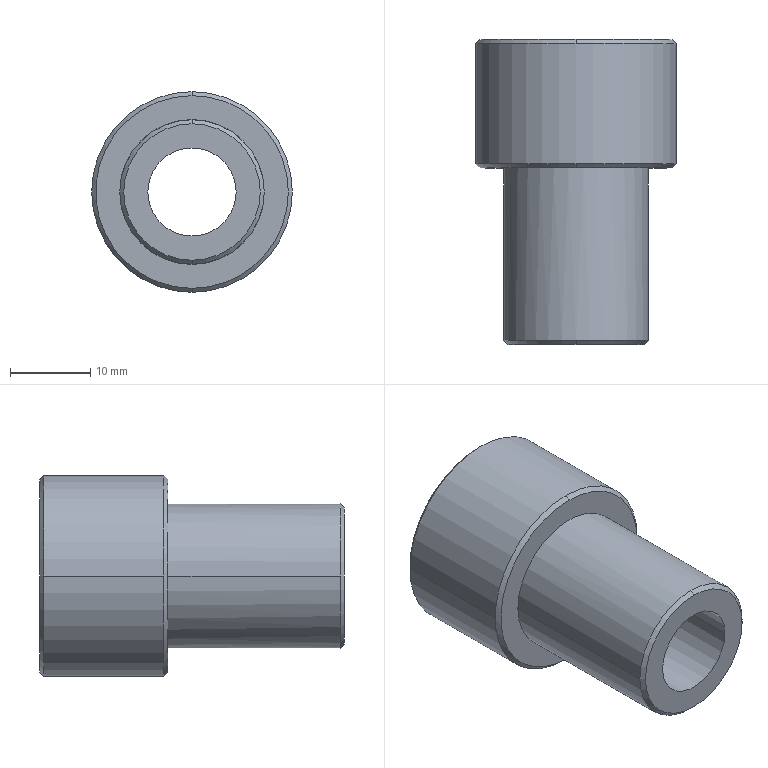Part | Creo | 1 solid | 20 faces | box 25 x 38 x 25 mm | volume 8054 mm3 | cylinder 8 | cone 8 | plane 4 | commonest cylinder face diameters 18 x4 11 x2 25 x2
STEP:
#1=CARTESIAN_POINT('',(-198.,355.995,-140.));
#2=VERTEX_POINT('',#1);
#3=CARTESIAN_POINT('',(-187.,355.995,-140.));
#4=VERTEX_POINT('',#3);
#5=CARTESIAN_POINT('',(-192.5,355.995,-140.));
#6=DIRECTION('',(0.,-1.,0.));
#7=DIRECTION('',(-1.,0.,0.));
#8=AXIS2_PLACEMENT_3D('',#5,#6,#7);
#9=CIRCLE('',#8,5.5);
#10=EDGE_CURVE('',#2,#4,#9,.T.);
#11=ORIENTED_EDGE('',*,*,#10,.T.);
#12=CARTESIAN_POINT('',(-187.,328.995,-140.));
#13=VERTEX_POINT('',#12);
#14=CARTESIAN_POINT('',(-187.,328.995,-140.));
#15=DIRECTION('',(0.,1.,0.));
#16=VECTOR('',#15,27.);
#17=LINE('',#14,#16);
#18=EDGE_CURVE('',#13,#4,#17,.T.);
#19=ORIENTED_EDGE('',*,*,#18,.F.);
#20=CARTESIAN_POINT('',(-198.,328.995,-140.));
#21=VERTEX_POINT('',#20);
#22=CARTESIAN_POINT('',(-192.5,328.995,-140.));
#23=DIRECTION('',(0.,1.,0.));
#24=DIRECTION('',(1.,0.,0.));
#25=AXIS2_PLACEMENT_3D('',#22,#23,#24);
#26=CIRCLE('',#25,5.5);
#27=EDGE_CURVE('',#13,#21,#26,.T.);
#28=ORIENTED_EDGE('',*,*,#27,.T.);
#29=CARTESIAN_POINT('',(-198.,328.995,-140.));
#30=DIRECTION('',(0.,1.,0.));
#31=VECTOR('',#30,27.);
#32=LINE('',#29,#31);
#33=EDGE_CURVE('',#21,#2,#32,.T.);
#34=ORIENTED_EDGE('',*,*,#33,.T.);
#35=EDGE_LOOP('',(#11,#19,#28,#34));
#36=FACE_OUTER_BOUND('',#35,.F.);
#37=CARTESIAN_POINT('',(-192.5,355.995,-140.));
#38=DIRECTION('',(0.,1.,0.));
#39=DIRECTION('',(1.,0.,0.));
#40=AXIS2_PLACEMENT_3D('',#37,#38,#39);
#41=CYLINDRICAL_SURFACE('',#40,5.5);
#42=ADVANCED_FACE('',(#36),#41,.F.);
#43=CARTESIAN_POINT('',(-183.5,355.995,-140.));
#44=VERTEX_POINT('',#43);
#45=CARTESIAN_POINT('',(-201.5,355.995,-140.));
#46=VERTEX_POINT('',#45);
#47=CARTESIAN_POINT('',(-192.5,355.995,-140.));
#48=DIRECTION('',(0.,1.,0.));
#49=DIRECTION('',(1.,0.,0.));
#50=AXIS2_PLACEMENT_3D('',#47,#48,#49);
#51=CIRCLE('',#50,9.);
#52=EDGE_CURVE('',#44,#46,#51,.T.);
#53=ORIENTED_EDGE('',*,*,#52,.F.);
#54=CARTESIAN_POINT('',(-192.5,355.995,-140.));
#55=DIRECTION('',(0.,1.,0.));
#56=DIRECTION('',(-1.,0.,0.));
#57=AXIS2_PLACEMENT_3D('',#54,#55,#56);
#58=CIRCLE('',#57,9.);
#59=EDGE_CURVE('',#46,#44,#58,.T.);
#60=ORIENTED_EDGE('',*,*,#59,.F.);
#61=EDGE_LOOP('',(#53,#60));
#62=FACE_OUTER_BOUND('',#61,.F.);
#63=CARTESIAN_POINT('',(-192.5,355.995,-140.));
#64=DIRECTION('',(0.,-1.,0.));
#65=DIRECTION('',(1.,0.,0.));
#66=AXIS2_PLACEMENT_3D('',#63,#64,#65);
#67=CIRCLE('',#66,5.5);
#68=EDGE_CURVE('',#4,#2,#67,.T.);
#69=ORIENTED_EDGE('',*,*,#68,.F.);
#70=ORIENTED_EDGE('',*,*,#10,.F.);
#71=EDGE_LOOP('',(#69,#70));
#72=FACE_BOUND('',#71,.F.);
#73=CARTESIAN_POINT('',(-192.5,355.995,-140.));
#74=DIRECTION('',(0.,-1.,0.));
#75=DIRECTION('',(1.,0.,0.));
#76=AXIS2_PLACEMENT_3D('',#73,#74,#75);
#77=PLANE('',#76);
#78=ADVANCED_FACE('',(#62,#72),#77,.F.);
#79=ORIENTED_EDGE('',*,*,#68,.T.);
#80=ORIENTED_EDGE('',*,*,#33,.F.);
#81=CARTESIAN_POINT('',(-192.5,328.995,-140.));
#82=DIRECTION('',(0.,1.,0.));
#83=DIRECTION('',(-1.,0.,0.));
#84=AXIS2_PLACEMENT_3D('',#81,#82,#83);
#85=CIRCLE('',#84,5.5);
#86=EDGE_CURVE('',#21,#13,#85,.T.);
#87=ORIENTED_EDGE('',*,*,#86,.T.);
#88=ORIENTED_EDGE('',*,*,#18,.T.);
#89=EDGE_LOOP('',(#79,#80,#87,#88));
#90=FACE_OUTER_BOUND('',#89,.F.);
#91=CARTESIAN_POINT('',(-192.5,355.995,-140.));
#92=DIRECTION('',(0.,1.,0.));
#93=DIRECTION('',(1.,0.,0.));
#94=AXIS2_PLACEMENT_3D('',#91,#92,#93);
#95=CYLINDRICAL_SURFACE('',#94,5.5);
#96=ADVANCED_FACE('',(#90),#95,.F.);
#97=CARTESIAN_POINT('',(-201.,328.995,-140.));
#98=VERTEX_POINT('',#97);
#99=CARTESIAN_POINT('',(-192.5,328.995,-148.5));
#100=VERTEX_POINT('',#99);
#101=CARTESIAN_POINT('',(-192.5,328.995,-140.));
#102=DIRECTION('',(0.,-1.,0.));
#103=DIRECTION('',(-1.,0.,0.));
#104=AXIS2_PLACEMENT_3D('',#101,#102,#103);
#105=CIRCLE('',#104,8.5);
#106=EDGE_CURVE('',#98,#100,#105,.T.);
#107=ORIENTED_EDGE('',*,*,#106,.F.);
#108=CARTESIAN_POINT('',(-192.5,328.995,-131.5));
#109=VERTEX_POINT('',#108);
#110=CARTESIAN_POINT('',(-192.5,328.995,-140.));
#111=DIRECTION('',(0.,-1.,0.));
#112=DIRECTION('',(0.,0.,1.));
#113=AXIS2_PLACEMENT_3D('',#110,#111,#112);
#114=CIRCLE('',#113,8.5);
#115=EDGE_CURVE('',#109,#98,#114,.T.);
#116=ORIENTED_EDGE('',*,*,#115,.F.);
#117=CARTESIAN_POINT('',(-184.,328.995,-140.));
#118=VERTEX_POINT('',#117);
#119=CARTESIAN_POINT('',(-192.5,328.995,-140.));
#120=DIRECTION('',(0.,-1.,0.));
#121=DIRECTION('',(1.,0.,0.));
#122=AXIS2_PLACEMENT_3D('',#119,#120,#121);
#123=CIRCLE('',#122,8.5);
#124=EDGE_CURVE('',#118,#109,#123,.T.);
#125=ORIENTED_EDGE('',*,*,#124,.F.);
#126=CARTESIAN_POINT('',(-192.5,328.995,-140.));
#127=DIRECTION('',(0.,-1.,0.));
#128=DIRECTION('',(0.,0.,-1.));
#129=AXIS2_PLACEMENT_3D('',#126,#127,#128);
#130=CIRCLE('',#129,8.5);
#131=EDGE_CURVE('',#100,#118,#130,.T.);
#132=ORIENTED_EDGE('',*,*,#131,.F.);
#133=EDGE_LOOP('',(#107,#116,#125,#132));
#134=FACE_OUTER_BOUND('',#133,.F.);
#135=ORIENTED_EDGE('',*,*,#27,.F.);
#136=ORIENTED_EDGE('',*,*,#86,.F.);
#137=EDGE_LOOP('',(#135,#136));
#138=FACE_BOUND('',#137,.F.);
#139=CARTESIAN_POINT('',(-232.5,328.995,-10.));
#140=DIRECTION('',(0.,-1.,0.));
#141=DIRECTION('',(1.,0.,0.));
#142=AXIS2_PLACEMENT_3D('',#139,#140,#141);
#143=PLANE('',#142);
#144=ADVANCED_FACE('',(#134,#138),#143,.T.);
#145=CARTESIAN_POINT('',(-201.5,329.495,-140.));
#146=VERTEX_POINT('',#145);
#147=CARTESIAN_POINT('',(-192.5,329.495,-149.));
#148=VERTEX_POINT('',#147);
#149=CARTESIAN_POINT('',(-192.5,329.495,-140.));
#150=DIRECTION('',(0.,-1.,0.));
#151=DIRECTION('',(-1.,0.,0.));
#152=AXIS2_PLACEMENT_3D('',#149,#150,#151);
#153=CIRCLE('',#152,9.);
#154=EDGE_CURVE('',#146,#148,#153,.T.);
#155=ORIENTED_EDGE('',*,*,#154,.F.);
#156=CARTESIAN_POINT('',(-192.5,329.495,-131.));
#157=VERTEX_POINT('',#156);
#158=CARTESIAN_POINT('',(-192.5,329.495,-140.));
#159=DIRECTION('',(0.,-1.,0.));
#160=DIRECTION('',(0.,0.,1.));
#161=AXIS2_PLACEMENT_3D('',#158,#159,#160);
#162=CIRCLE('',#161,9.);
#163=EDGE_CURVE('',#157,#146,#162,.T.);
#164=ORIENTED_EDGE('',*,*,#163,.F.);
#165=CARTESIAN_POINT('',(-192.5,328.995,-131.5));
#166=DIRECTION('',(0.,0.7071,0.7071));
#167=VECTOR('',#166,0.7071);
#168=LINE('',#165,#167);
#169=EDGE_CURVE('',#109,#157,#168,.T.);
#170=ORIENTED_EDGE('',*,*,#169,.F.);
#171=ORIENTED_EDGE('',*,*,#115,.T.);
#172=ORIENTED_EDGE('',*,*,#106,.T.);
#173=CARTESIAN_POINT('',(-192.5,328.995,-148.5));
#174=DIRECTION('',(0.,0.7071,-0.7071));
#175=VECTOR('',#174,0.7071);
#176=LINE('',#173,#175);
#177=EDGE_CURVE('',#100,#148,#176,.T.);
#178=ORIENTED_EDGE('',*,*,#177,.T.);
#179=EDGE_LOOP('',(#155,#164,#170,#171,#172,#178));
#180=FACE_OUTER_BOUND('',#179,.F.);
#181=CARTESIAN_POINT('',(-192.5,329.245,-140.));
#182=DIRECTION('',(0.,1.,0.));
#183=DIRECTION('',(0.,0.,-1.));
#184=AXIS2_PLACEMENT_3D('',#181,#182,#183);
#185=CONICAL_SURFACE('',#184,8.75,45.);
#186=ADVANCED_FACE('',(#180),#185,.T.);
#187=CARTESIAN_POINT('',(-183.5,329.495,-140.));
#188=VERTEX_POINT('',#187);
#189=CARTESIAN_POINT('',(-192.5,329.495,-140.));
#190=DIRECTION('',(0.,-1.,0.));
#191=DIRECTION('',(0.,0.,-1.));
#192=AXIS2_PLACEMENT_3D('',#189,#190,#191);
#193=CIRCLE('',#192,9.);
#194=EDGE_CURVE('',#148,#188,#193,.T.);
#195=ORIENTED_EDGE('',*,*,#194,.T.);
#196=CARTESIAN_POINT('',(-183.5,350.995,-140.));
#197=VERTEX_POINT('',#196);
#198=CARTESIAN_POINT('',(-183.5,350.995,-140.));
#199=DIRECTION('',(0.,-1.,0.));
#200=VECTOR('',#199,21.5);
#201=LINE('',#198,#200);
#202=EDGE_CURVE('',#197,#188,#201,.T.);
#203=ORIENTED_EDGE('',*,*,#202,.F.);
#204=CARTESIAN_POINT('',(-201.5,350.995,-140.));
#205=VERTEX_POINT('',#204);
#206=CARTESIAN_POINT('',(-192.5,350.995,-140.));
#207=DIRECTION('',(0.,1.,0.));
#208=DIRECTION('',(1.,0.,0.));
#209=AXIS2_PLACEMENT_3D('',#206,#207,#208);
#210=CIRCLE('',#209,9.);
#211=EDGE_CURVE('',#197,#205,#210,.T.);
#212=ORIENTED_EDGE('',*,*,#211,.T.);
#213=CARTESIAN_POINT('',(-201.5,350.995,-140.));
#214=DIRECTION('',(0.,-1.,0.));
#215=VECTOR('',#214,21.5);
#216=LINE('',#213,#215);
#217=EDGE_CURVE('',#205,#146,#216,.T.);
#218=ORIENTED_EDGE('',*,*,#217,.T.);
#219=ORIENTED_EDGE('',*,*,#154,.T.);
#220=EDGE_LOOP('',(#195,#203,#212,#218,#219));
#221=FACE_OUTER_BOUND('',#220,.F.);
#222=CARTESIAN_POINT('',(-192.5,331.995,-140.));
#223=DIRECTION('',(0.,-1.,0.));
#224=DIRECTION('',(1.,0.,0.));
#225=AXIS2_PLACEMENT_3D('',#222,#223,#224);
#226=CYLINDRICAL_SURFACE('',#225,9.);
#227=ADVANCED_FACE('',(#221),#226,.T.);
#228=ORIENTED_EDGE('',*,*,#194,.F.);
#229=ORIENTED_EDGE('',*,*,#177,.F.);
#230=ORIENTED_EDGE('',*,*,#131,.T.);
#231=ORIENTED_EDGE('',*,*,#124,.T.);
#232=ORIENTED_EDGE('',*,*,#169,.T.);
#233=CARTESIAN_POINT('',(-192.5,329.495,-140.));
#234=DIRECTION('',(0.,-1.,0.));
#235=DIRECTION('',(1.,0.,0.));
#236=AXIS2_PLACEMENT_3D('',#233,#234,#235);
#237=CIRCLE('',#236,9.);
#238=EDGE_CURVE('',#188,#157,#237,.T.);
#239=ORIENTED_EDGE('',*,*,#238,.F.);
#240=EDGE_LOOP('',(#228,#229,#230,#231,#232,#239));
#241=FACE_OUTER_BOUND('',#240,.F.);
#242=CARTESIAN_POINT('',(-192.5,329.245,-140.));
#243=DIRECTION('',(0.,1.,0.));
#244=DIRECTION('',(0.,0.,-1.));
#245=AXIS2_PLACEMENT_3D('',#242,#243,#244);
#246=CONICAL_SURFACE('',#245,8.75,45.);
#247=ADVANCED_FACE('',(#241),#246,.T.);
#248=ORIENTED_EDGE('',*,*,#163,.T.);
#249=ORIENTED_EDGE('',*,*,#217,.F.);
#250=CARTESIAN_POINT('',(-192.5,350.995,-140.));
#251=DIRECTION('',(0.,1.,0.));
#252=DIRECTION('',(-1.,0.,0.));
#253=AXIS2_PLACEMENT_3D('',#250,#251,#252);
#254=CIRCLE('',#253,9.);
#255=EDGE_CURVE('',#205,#197,#254,.T.);
#256=ORIENTED_EDGE('',*,*,#255,.T.);
#257=ORIENTED_EDGE('',*,*,#202,.T.);
#258=ORIENTED_EDGE('',*,*,#238,.T.);
#259=EDGE_LOOP('',(#248,#249,#256,#257,#258));
#260=FACE_OUTER_BOUND('',#259,.F.);
#261=CARTESIAN_POINT('',(-192.5,331.995,-140.));
#262=DIRECTION('',(0.,-1.,0.));
#263=DIRECTION('',(1.,0.,0.));
#264=AXIS2_PLACEMENT_3D('',#261,#262,#263);
#265=CYLINDRICAL_SURFACE('',#264,9.);
#266=ADVANCED_FACE('',(#260),#265,.T.);
#267=CARTESIAN_POINT('',(-180.5,350.995,-140.));
#268=VERTEX_POINT('',#267);
#269=CARTESIAN_POINT('',(-192.5,350.995,-128.));
#270=VERTEX_POINT('',#269);
#271=CARTESIAN_POINT('',(-192.5,350.995,-140.));
#272=DIRECTION('',(0.,-1.,0.));
#273=DIRECTION('',(1.,0.,0.));
#274=AXIS2_PLACEMENT_3D('',#271,#272,#273);
#275=CIRCLE('',#274,12.);
#276=EDGE_CURVE('',#268,#270,#275,.T.);
#277=ORIENTED_EDGE('',*,*,#276,.F.);
#278=CARTESIAN_POINT('',(-192.5,350.995,-152.));
#279=VERTEX_POINT('',#278);
#280=CARTESIAN_POINT('',(-192.5,350.995,-140.));
#281=DIRECTION('',(0.,-1.,0.));
#282=DIRECTION('',(0.,0.,-1.));
#283=AXIS2_PLACEMENT_3D('',#280,#281,#282);
#284=CIRCLE('',#283,12.);
#285=EDGE_CURVE('',#279,#268,#284,.T.);
#286=ORIENTED_EDGE('',*,*,#285,.F.);
#287=CARTESIAN_POINT('',(-192.5,350.995,-140.));
#288=DIRECTION('',(0.,-1.,0.));
#289=DIRECTION('',(0.,0.,1.));
#290=AXIS2_PLACEMENT_3D('',#287,#288,#289);
#291=CIRCLE('',#290,12.);
#292=EDGE_CURVE('',#270,#279,#291,.T.);
#293=ORIENTED_EDGE('',*,*,#292,.F.);
#294=EDGE_LOOP('',(#277,#286,#293));
#295=FACE_OUTER_BOUND('',#294,.F.);
#296=ORIENTED_EDGE('',*,*,#255,.F.);
#297=ORIENTED_EDGE('',*,*,#211,.F.);
#298=EDGE_LOOP('',(#296,#297));
#299=FACE_BOUND('',#298,.F.);
#300=CARTESIAN_POINT('',(-232.5,350.995,-10.));
#301=DIRECTION('',(0.,-1.,0.));
#302=DIRECTION('',(1.,0.,0.));
#303=AXIS2_PLACEMENT_3D('',#300,#301,#302);
#304=PLANE('',#303);
#305=ADVANCED_FACE('',(#295,#299),#304,.T.);
#306=CARTESIAN_POINT('',(-180.,351.495,-140.));
#307=VERTEX_POINT('',#306);
#308=CARTESIAN_POINT('',(-192.5,351.495,-127.5));
#309=VERTEX_POINT('',#308);
#310=CARTESIAN_POINT('',(-192.5,351.495,-140.));
#311=DIRECTION('',(0.,-1.,0.));
#312=DIRECTION('',(1.,0.,0.));
#313=AXIS2_PLACEMENT_3D('',#310,#311,#312);
#314=CIRCLE('',#313,12.5);
#315=EDGE_CURVE('',#307,#309,#314,.T.);
#316=ORIENTED_EDGE('',*,*,#315,.F.);
#317=CARTESIAN_POINT('',(-192.5,351.495,-152.5));
#318=VERTEX_POINT('',#317);
#319=CARTESIAN_POINT('',(-192.5,351.495,-140.));
#320=DIRECTION('',(0.,-1.,0.));
#321=DIRECTION('',(0.,0.,-1.));
#322=AXIS2_PLACEMENT_3D('',#319,#320,#321);
#323=CIRCLE('',#322,12.5);
#324=EDGE_CURVE('',#318,#307,#323,.T.);
#325=ORIENTED_EDGE('',*,*,#324,.F.);
#326=CARTESIAN_POINT('',(-192.5,350.995,-152.));
#327=DIRECTION('',(0.,0.7071,-0.7071));
#328=VECTOR('',#327,0.7071);
#329=LINE('',#326,#328);
#330=EDGE_CURVE('',#279,#318,#329,.T.);
#331=ORIENTED_EDGE('',*,*,#330,.F.);
#332=ORIENTED_EDGE('',*,*,#285,.T.);
#333=ORIENTED_EDGE('',*,*,#276,.T.);
#334=CARTESIAN_POINT('',(-192.5,350.995,-128.));
#335=DIRECTION('',(0.,0.7071,0.7071));
#336=VECTOR('',#335,0.7071);
#337=LINE('',#334,#336);
#338=EDGE_CURVE('',#270,#309,#337,.T.);
#339=ORIENTED_EDGE('',*,*,#338,.T.);
#340=EDGE_LOOP('',(#316,#325,#331,#332,#333,#339));
#341=FACE_OUTER_BOUND('',#340,.F.);
#342=CARTESIAN_POINT('',(-192.5,351.245,-140.));
#343=DIRECTION('',(0.,1.,0.));
#344=DIRECTION('',(0.,0.,-1.));
#345=AXIS2_PLACEMENT_3D('',#342,#343,#344);
#346=CONICAL_SURFACE('',#345,12.25,45.);
#347=ADVANCED_FACE('',(#341),#346,.T.);
#348=CARTESIAN_POINT('',(-205.,351.495,-140.));
#349=VERTEX_POINT('',#348);
#350=CARTESIAN_POINT('',(-192.5,351.495,-140.));
#351=DIRECTION('',(0.,-1.,0.));
#352=DIRECTION('',(0.,0.,1.));
#353=AXIS2_PLACEMENT_3D('',#350,#351,#352);
#354=CIRCLE('',#353,12.5);
#355=EDGE_CURVE('',#309,#349,#354,.T.);
#356=ORIENTED_EDGE('',*,*,#355,.T.);
#357=CARTESIAN_POINT('',(-205.,366.495,-140.));
#358=VERTEX_POINT('',#357);
#359=CARTESIAN_POINT('',(-205.,366.495,-140.));
#360=DIRECTION('',(0.,-1.,0.));
#361=VECTOR('',#360,15.);
#362=LINE('',#359,#361);
#363=EDGE_CURVE('',#358,#349,#362,.T.);
#364=ORIENTED_EDGE('',*,*,#363,.F.);
#365=CARTESIAN_POINT('',(-192.5,366.495,-127.5));
#366=VERTEX_POINT('',#365);
#367=CARTESIAN_POINT('',(-192.5,366.495,-140.));
#368=DIRECTION('',(0.,1.,0.));
#369=DIRECTION('',(-1.,0.,0.));
#370=AXIS2_PLACEMENT_3D('',#367,#368,#369);
#371=CIRCLE('',#370,12.5);
#372=EDGE_CURVE('',#358,#366,#371,.T.);
#373=ORIENTED_EDGE('',*,*,#372,.T.);
#374=CARTESIAN_POINT('',(-180.,366.495,-140.));
#375=VERTEX_POINT('',#374);
#376=CARTESIAN_POINT('',(-192.5,366.495,-140.));
#377=DIRECTION('',(0.,1.,0.));
#378=DIRECTION('',(0.,0.,1.));
#379=AXIS2_PLACEMENT_3D('',#376,#377,#378);
#380=CIRCLE('',#379,12.5);
#381=EDGE_CURVE('',#366,#375,#380,.T.);
#382=ORIENTED_EDGE('',*,*,#381,.T.);
#383=CARTESIAN_POINT('',(-180.,366.495,-140.));
#384=DIRECTION('',(0.,-1.,0.));
#385=VECTOR('',#384,15.);
#386=LINE('',#383,#385);
#387=EDGE_CURVE('',#375,#307,#386,.T.);
#388=ORIENTED_EDGE('',*,*,#387,.T.);
#389=ORIENTED_EDGE('',*,*,#315,.T.);
#390=EDGE_LOOP('',(#356,#364,#373,#382,#388,#389));
#391=FACE_OUTER_BOUND('',#390,.F.);
#392=CARTESIAN_POINT('',(-192.5,331.995,-140.));
#393=DIRECTION('',(0.,-1.,0.));
#394=DIRECTION('',(1.,0.,0.));
#395=AXIS2_PLACEMENT_3D('',#392,#393,#394);
#396=CYLINDRICAL_SURFACE('',#395,12.5);
#397=ADVANCED_FACE('',(#391),#396,.T.);
#398=ORIENTED_EDGE('',*,*,#355,.F.);
#399=ORIENTED_EDGE('',*,*,#338,.F.);
#400=ORIENTED_EDGE('',*,*,#292,.T.);
#401=ORIENTED_EDGE('',*,*,#330,.T.);
#402=CARTESIAN_POINT('',(-192.5,351.495,-140.));
#403=DIRECTION('',(0.,-1.,0.));
#404=DIRECTION('',(-1.,0.,0.));
#405=AXIS2_PLACEMENT_3D('',#402,#403,#404);
#406=CIRCLE('',#405,12.5);
#407=EDGE_CURVE('',#349,#318,#406,.T.);
#408=ORIENTED_EDGE('',*,*,#407,.F.);
#409=EDGE_LOOP('',(#398,#399,#400,#401,#408));
#410=FACE_OUTER_BOUND('',#409,.F.);
#411=CARTESIAN_POINT('',(-192.5,351.245,-140.));
#412=DIRECTION('',(0.,1.,0.));
#413=DIRECTION('',(0.,0.,-1.));
#414=AXIS2_PLACEMENT_3D('',#411,#412,#413);
#415=CONICAL_SURFACE('',#414,12.25,45.);
#416=ADVANCED_FACE('',(#410),#415,.T.);
#417=ORIENTED_EDGE('',*,*,#324,.T.);
#418=ORIENTED_EDGE('',*,*,#387,.F.);
#419=CARTESIAN_POINT('',(-192.5,366.495,-152.5));
#420=VERTEX_POINT('',#419);
#421=CARTESIAN_POINT('',(-192.5,366.495,-140.));
#422=DIRECTION('',(0.,1.,0.));
#423=DIRECTION('',(1.,0.,0.));
#424=AXIS2_PLACEMENT_3D('',#421,#422,#423);
#425=CIRCLE('',#424,12.5);
#426=EDGE_CURVE('',#375,#420,#425,.T.);
#427=ORIENTED_EDGE('',*,*,#426,.T.);
#428=CARTESIAN_POINT('',(-192.5,366.495,-140.));
#429=DIRECTION('',(0.,1.,0.));
#430=DIRECTION('',(0.,0.,-1.));
#431=AXIS2_PLACEMENT_3D('',#428,#429,#430);
#432=CIRCLE('',#431,12.5);
#433=EDGE_CURVE('',#420,#358,#432,.T.);
#434=ORIENTED_EDGE('',*,*,#433,.T.);
#435=ORIENTED_EDGE('',*,*,#363,.T.);
#436=ORIENTED_EDGE('',*,*,#407,.T.);
#437=EDGE_LOOP('',(#417,#418,#427,#434,#435,#436));
#438=FACE_OUTER_BOUND('',#437,.F.);
#439=CARTESIAN_POINT('',(-192.5,331.995,-140.));
#440=DIRECTION('',(0.,-1.,0.));
#441=DIRECTION('',(1.,0.,0.));
#442=AXIS2_PLACEMENT_3D('',#439,#440,#441);
#443=CYLINDRICAL_SURFACE('',#442,12.5);
#444=ADVANCED_FACE('',(#438),#443,.T.);
#445=CARTESIAN_POINT('',(-192.5,366.995,-128.));
#446=VERTEX_POINT('',#445);
#447=CARTESIAN_POINT('',(-180.5,366.995,-140.));
#448=VERTEX_POINT('',#447);
#449=CARTESIAN_POINT('',(-192.5,366.995,-140.));
#450=DIRECTION('',(0.,1.,0.));
#451=DIRECTION('',(0.,0.,1.));
#452=AXIS2_PLACEMENT_3D('',#449,#450,#451);
#453=CIRCLE('',#452,12.);
#454=EDGE_CURVE('',#446,#448,#453,.T.);
#455=ORIENTED_EDGE('',*,*,#454,.T.);
#456=CARTESIAN_POINT('',(-192.5,366.995,-152.));
#457=VERTEX_POINT('',#456);
#458=CARTESIAN_POINT('',(-192.5,366.995,-140.));
#459=DIRECTION('',(0.,1.,0.));
#460=DIRECTION('',(1.,0.,0.));
#461=AXIS2_PLACEMENT_3D('',#458,#459,#460);
#462=CIRCLE('',#461,12.);
#463=EDGE_CURVE('',#448,#457,#462,.T.);
#464=ORIENTED_EDGE('',*,*,#463,.T.);
#465=CARTESIAN_POINT('',(-192.5,366.995,-152.));
#466=DIRECTION('',(0.,-0.7071,-0.7071));
#467=VECTOR('',#466,0.7071);
#468=LINE('',#465,#467);
#469=EDGE_CURVE('',#457,#420,#468,.T.);
#470=ORIENTED_EDGE('',*,*,#469,.T.);
#471=ORIENTED_EDGE('',*,*,#426,.F.);
#472=ORIENTED_EDGE('',*,*,#381,.F.);
#473=CARTESIAN_POINT('',(-192.5,366.995,-128.));
#474=DIRECTION('',(0.,-0.7071,0.7071));
#475=VECTOR('',#474,0.7071);
#476=LINE('',#473,#475);
#477=EDGE_CURVE('',#446,#366,#476,.T.);
#478=ORIENTED_EDGE('',*,*,#477,.F.);
#479=EDGE_LOOP('',(#455,#464,#470,#471,#472,#478));
#480=FACE_OUTER_BOUND('',#479,.F.);
#481=CARTESIAN_POINT('',(-192.5,366.745,-140.));
#482=DIRECTION('',(0.,-1.,0.));
#483=DIRECTION('',(0.,0.,-1.));
#484=AXIS2_PLACEMENT_3D('',#481,#482,#483);
#485=CONICAL_SURFACE('',#484,12.25,45.);
#486=ADVANCED_FACE('',(#480),#485,.T.);
#487=ORIENTED_EDGE('',*,*,#463,.F.);
#488=ORIENTED_EDGE('',*,*,#454,.F.);
#489=CARTESIAN_POINT('',(-204.5,366.995,-140.));
#490=VERTEX_POINT('',#489);
#491=CARTESIAN_POINT('',(-192.5,366.995,-140.));
#492=DIRECTION('',(0.,1.,0.));
#493=DIRECTION('',(-1.,0.,0.));
#494=AXIS2_PLACEMENT_3D('',#491,#492,#493);
#495=CIRCLE('',#494,12.);
#496=EDGE_CURVE('',#490,#446,#495,.T.);
#497=ORIENTED_EDGE('',*,*,#496,.F.);
#498=CARTESIAN_POINT('',(-192.5,366.995,-140.));
#499=DIRECTION('',(0.,1.,0.));
#500=DIRECTION('',(0.,0.,-1.));
#501=AXIS2_PLACEMENT_3D('',#498,#499,#500);
#502=CIRCLE('',#501,12.);
#503=EDGE_CURVE('',#457,#490,#502,.T.);
#504=ORIENTED_EDGE('',*,*,#503,.F.);
#505=EDGE_LOOP('',(#487,#488,#497,#504));
#506=FACE_OUTER_BOUND('',#505,.F.);
#507=CARTESIAN_POINT('',(-202.,366.995,-140.));
#508=VERTEX_POINT('',#507);
#509=CARTESIAN_POINT('',(-192.5,366.995,-149.5));
#510=VERTEX_POINT('',#509);
#511=CARTESIAN_POINT('',(-192.5,366.995,-140.));
#512=DIRECTION('',(0.,-1.,0.));
#513=DIRECTION('',(-1.,0.,0.));
#514=AXIS2_PLACEMENT_3D('',#511,#512,#513);
#515=CIRCLE('',#514,9.5);
#516=EDGE_CURVE('',#508,#510,#515,.T.);
#517=ORIENTED_EDGE('',*,*,#516,.F.);
#518=CARTESIAN_POINT('',(-192.5,366.995,-130.5));
#519=VERTEX_POINT('',#518);
#520=CARTESIAN_POINT('',(-192.5,366.995,-140.));
#521=DIRECTION('',(0.,-1.,0.));
#522=DIRECTION('',(0.,0.,1.));
#523=AXIS2_PLACEMENT_3D('',#520,#521,#522);
#524=CIRCLE('',#523,9.5);
#525=EDGE_CURVE('',#519,#508,#524,.T.);
#526=ORIENTED_EDGE('',*,*,#525,.F.);
#527=CARTESIAN_POINT('',(-183.,366.995,-140.));
#528=VERTEX_POINT('',#527);
#529=CARTESIAN_POINT('',(-192.5,366.995,-140.));
#530=DIRECTION('',(0.,-1.,0.));
#531=DIRECTION('',(1.,0.,0.));
#532=AXIS2_PLACEMENT_3D('',#529,#530,#531);
#533=CIRCLE('',#532,9.5);
#534=EDGE_CURVE('',#528,#519,#533,.T.);
#535=ORIENTED_EDGE('',*,*,#534,.F.);
#536=CARTESIAN_POINT('',(-192.5,366.995,-140.));
#537=DIRECTION('',(0.,-1.,0.));
#538=DIRECTION('',(0.,0.,-1.));
#539=AXIS2_PLACEMENT_3D('',#536,#537,#538);
#540=CIRCLE('',#539,9.5);
#541=EDGE_CURVE('',#510,#528,#540,.T.);
#542=ORIENTED_EDGE('',*,*,#541,.F.);
#543=EDGE_LOOP('',(#517,#526,#535,#542));
#544=FACE_BOUND('',#543,.F.);
#545=CARTESIAN_POINT('',(-232.5,366.995,-10.));
#546=DIRECTION('',(0.,-1.,0.));
#547=DIRECTION('',(1.,0.,0.));
#548=AXIS2_PLACEMENT_3D('',#545,#546,#547);
#549=PLANE('',#548);
#550=ADVANCED_FACE('',(#506,#544),#549,.F.);
#551=CARTESIAN_POINT('',(-201.5,366.495,-140.));
#552=VERTEX_POINT('',#551);
#553=CARTESIAN_POINT('',(-192.5,366.495,-149.));
#554=VERTEX_POINT('',#553);
#555=CARTESIAN_POINT('',(-192.5,366.495,-140.));
#556=DIRECTION('',(0.,-1.,0.));
#557=DIRECTION('',(-1.,0.,0.));
#558=AXIS2_PLACEMENT_3D('',#555,#556,#557);
#559=CIRCLE('',#558,9.);
#560=EDGE_CURVE('',#552,#554,#559,.T.);
#561=ORIENTED_EDGE('',*,*,#560,.F.);
#562=CARTESIAN_POINT('',(-192.5,366.495,-131.));
#563=VERTEX_POINT('',#562);
#564=CARTESIAN_POINT('',(-192.5,366.495,-140.));
#565=DIRECTION('',(0.,-1.,0.));
#566=DIRECTION('',(0.,0.,1.));
#567=AXIS2_PLACEMENT_3D('',#564,#565,#566);
#568=CIRCLE('',#567,9.);
#569=EDGE_CURVE('',#563,#552,#568,.T.);
#570=ORIENTED_EDGE('',*,*,#569,.F.);
#571=CARTESIAN_POINT('',(-192.5,366.495,-131.));
#572=DIRECTION('',(0.,0.7071,0.7071));
#573=VECTOR('',#572,0.7071);
#574=LINE('',#571,#573);
#575=EDGE_CURVE('',#563,#519,#574,.T.);
#576=ORIENTED_EDGE('',*,*,#575,.T.);
#577=ORIENTED_EDGE('',*,*,#525,.T.);
#578=ORIENTED_EDGE('',*,*,#516,.T.);
#579=CARTESIAN_POINT('',(-192.5,366.495,-149.));
#580=DIRECTION('',(0.,0.7071,-0.7071));
#581=VECTOR('',#580,0.7071);
#582=LINE('',#579,#581);
#583=EDGE_CURVE('',#554,#510,#582,.T.);
#584=ORIENTED_EDGE('',*,*,#583,.F.);
#585=EDGE_LOOP('',(#561,#570,#576,#577,#578,#584));
#586=FACE_OUTER_BOUND('',#585,.F.);
#587=CARTESIAN_POINT('',(-192.5,366.745,-140.));
#588=DIRECTION('',(0.,1.,0.));
#589=DIRECTION('',(0.,0.,-1.));
#590=AXIS2_PLACEMENT_3D('',#587,#588,#589);
#591=CONICAL_SURFACE('',#590,9.25,45.);
#592=ADVANCED_FACE('',(#586),#591,.F.);
#593=CARTESIAN_POINT('',(-183.5,366.495,-140.));
#594=VERTEX_POINT('',#593);
#595=CARTESIAN_POINT('',(-192.5,366.495,-140.));
#596=DIRECTION('',(0.,-1.,0.));
#597=DIRECTION('',(0.,0.,-1.));
#598=AXIS2_PLACEMENT_3D('',#595,#596,#597);
#599=CIRCLE('',#598,9.);
#600=EDGE_CURVE('',#554,#594,#599,.T.);
#601=ORIENTED_EDGE('',*,*,#600,.T.);
#602=CARTESIAN_POINT('',(-183.5,366.495,-140.));
#603=DIRECTION('',(0.,-1.,0.));
#604=VECTOR('',#603,10.5);
#605=LINE('',#602,#604);
#606=EDGE_CURVE('',#594,#44,#605,.T.);
#607=ORIENTED_EDGE('',*,*,#606,.T.);
#608=ORIENTED_EDGE('',*,*,#52,.T.);
#609=CARTESIAN_POINT('',(-201.5,366.495,-140.));
#610=DIRECTION('',(0.,-1.,0.));
#611=VECTOR('',#610,10.5);
#612=LINE('',#609,#611);
#613=EDGE_CURVE('',#552,#46,#612,.T.);
#614=ORIENTED_EDGE('',*,*,#613,.F.);
#615=ORIENTED_EDGE('',*,*,#560,.T.);
#616=EDGE_LOOP('',(#601,#607,#608,#614,#615));
#617=FACE_OUTER_BOUND('',#616,.F.);
#618=CARTESIAN_POINT('',(-192.5,367.545,-140.));
#619=DIRECTION('',(0.,-1.,0.));
#620=DIRECTION('',(1.,0.,0.));
#621=AXIS2_PLACEMENT_3D('',#618,#619,#620);
#622=CYLINDRICAL_SURFACE('',#621,9.);
#623=ADVANCED_FACE('',(#617),#622,.F.);
#624=ORIENTED_EDGE('',*,*,#600,.F.);
#625=ORIENTED_EDGE('',*,*,#583,.T.);
#626=ORIENTED_EDGE('',*,*,#541,.T.);
#627=ORIENTED_EDGE('',*,*,#534,.T.);
#628=ORIENTED_EDGE('',*,*,#575,.F.);
#629=CARTESIAN_POINT('',(-192.5,366.495,-140.));
#630=DIRECTION('',(0.,-1.,0.));
#631=DIRECTION('',(1.,0.,0.));
#632=AXIS2_PLACEMENT_3D('',#629,#630,#631);
#633=CIRCLE('',#632,9.);
#634=EDGE_CURVE('',#594,#563,#633,.T.);
#635=ORIENTED_EDGE('',*,*,#634,.F.);
#636=EDGE_LOOP('',(#624,#625,#626,#627,#628,#635));
#637=FACE_OUTER_BOUND('',#636,.F.);
#638=CARTESIAN_POINT('',(-192.5,366.745,-140.));
#639=DIRECTION('',(0.,1.,0.));
#640=DIRECTION('',(0.,0.,-1.));
#641=AXIS2_PLACEMENT_3D('',#638,#639,#640);
#642=CONICAL_SURFACE('',#641,9.25,45.);
#643=ADVANCED_FACE('',(#637),#642,.F.);
#644=ORIENTED_EDGE('',*,*,#569,.T.);
#645=ORIENTED_EDGE('',*,*,#613,.T.);
#646=ORIENTED_EDGE('',*,*,#59,.T.);
#647=ORIENTED_EDGE('',*,*,#606,.F.);
#648=ORIENTED_EDGE('',*,*,#634,.T.);
#649=EDGE_LOOP('',(#644,#645,#646,#647,#648));
#650=FACE_OUTER_BOUND('',#649,.F.);
#651=CARTESIAN_POINT('',(-192.5,367.545,-140.));
#652=DIRECTION('',(0.,-1.,0.));
#653=DIRECTION('',(1.,0.,0.));
#654=AXIS2_PLACEMENT_3D('',#651,#652,#653);
#655=CYLINDRICAL_SURFACE('',#654,9.);
#656=ADVANCED_FACE('',(#650),#655,.F.);
#657=ORIENTED_EDGE('',*,*,#496,.T.);
#658=ORIENTED_EDGE('',*,*,#477,.T.);
#659=ORIENTED_EDGE('',*,*,#372,.F.);
#660=ORIENTED_EDGE('',*,*,#433,.F.);
#661=ORIENTED_EDGE('',*,*,#469,.F.);
#662=ORIENTED_EDGE('',*,*,#503,.T.);
#663=EDGE_LOOP('',(#657,#658,#659,#660,#661,#662));
#664=FACE_OUTER_BOUND('',#663,.F.);
#665=CARTESIAN_POINT('',(-192.5,366.745,-140.));
#666=DIRECTION('',(0.,-1.,0.));
#667=DIRECTION('',(0.,0.,-1.));
#668=AXIS2_PLACEMENT_3D('',#665,#666,#667);
#669=CONICAL_SURFACE('',#668,12.25,45.);
#670=ADVANCED_FACE('',(#664),#669,.T.);
#671=CLOSED_SHELL('',(#42,#78,#96,#144,#186,#227,#247,#266,#305,#347,#397,#416,#444,#486,#550,#592,#623,#643,#656,#670));
#672=MANIFOLD_SOLID_BREP('',#671);
#673=(LENGTH_UNIT()NAMED_UNIT(*)SI_UNIT(.MILLI.,.METRE.));
#674=UNCERTAINTY_MEASURE_WITH_UNIT(LENGTH_MEASURE(0.00519),#673,'','');
#675=(NAMED_UNIT(*)PLANE_ANGLE_UNIT()SI_UNIT($,.RADIAN.));
#676=PLANE_ANGLE_MEASURE_WITH_UNIT(PLANE_ANGLE_MEASURE(0.01745),#675);
#677=(CONVERSION_BASED_UNIT('DEGREE',#676)NAMED_UNIT(*)PLANE_ANGLE_UNIT());
#678=(NAMED_UNIT(*)SI_UNIT($,.STERADIAN.)SOLID_ANGLE_UNIT());
#679=(GEOMETRIC_REPRESENTATION_CONTEXT(3)GLOBAL_UNCERTAINTY_ASSIGNED_CONTEXT((#674))GLOBAL_UNIT_ASSIGNED_CONTEXT((#673,#677,#678))REPRESENTATION_CONTEXT('',''));
#680=ADVANCED_BREP_SHAPE_REPRESENTATION('',(#672),#679);